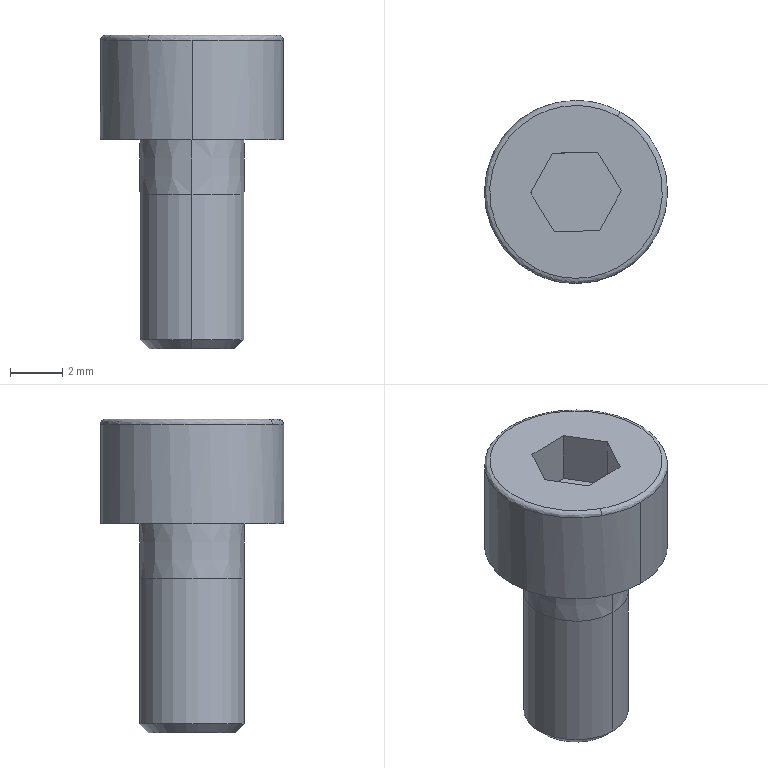Part | SolidWorks | features BaseBody 1 | 1 solid | 20 faces | box 7 x 7 x 12 mm | volume 237.96 mm3 | plane 10 | cylinder 4 | cone 4 | spline 2 | commonest cylinder face diameters 4 x2 7 x2
STEP:
#1=CARTESIAN_POINT('',(487.586,-57.42,293.048));
#2=VERTEX_POINT('',#1);
#3=CARTESIAN_POINT('',(489.266,-50.849,293.048));
#4=VERTEX_POINT('',#3);
#5=CARTESIAN_POINT('',(489.266,-54.349,293.048));
#6=DIRECTION('',(-0.000000004,0.000000009,-1.));
#7=DIRECTION('',(0.,1.,0.000000009));
#8=AXIS2_PLACEMENT_3D('',#5,#6,#7);
#9=CIRCLE('',#8,3.5);
#10=EDGE_CURVE('',#2,#4,#9,.T.);
#11=ORIENTED_EDGE('',*,*,#10,.F.);
#12=CARTESIAN_POINT('',(487.682,-57.244,293.248));
#13=VERTEX_POINT('',#12);
#14=CARTESIAN_POINT('',(487.682,-57.244,293.048));
#15=DIRECTION('',(-0.8773,0.4799,0.000000008));
#16=DIRECTION('',(-0.4799,-0.8773,-0.000000006));
#17=AXIS2_PLACEMENT_3D('',#14,#15,#16);
#18=CIRCLE('',#17,0.2);
#19=EDGE_CURVE('',#2,#13,#18,.T.);
#20=ORIENTED_EDGE('',*,*,#19,.T.);
#21=CARTESIAN_POINT('',(490.85,-51.454,293.248));
#22=VERTEX_POINT('',#21);
#23=CARTESIAN_POINT('',(487.682,-57.244,293.248));
#24=CARTESIAN_POINT('',(481.892,-54.077,293.248));
#25=CARTESIAN_POINT('',(485.059,-48.287,293.248));
#26=CARTESIAN_POINT('',(490.85,-51.454,293.248));
#27=(BOUNDED_CURVE()B_SPLINE_CURVE(3,(#23,#24,#25,#26),.UNSPECIFIED.,.F.,.F.)B_SPLINE_CURVE_WITH_KNOTS((4,4),(0.,1.),.UNSPECIFIED.)CURVE()GEOMETRIC_REPRESENTATION_ITEM()RATIONAL_B_SPLINE_CURVE((1.,0.3333,0.3333,1.))REPRESENTATION_ITEM(''));
#28=EDGE_CURVE('',#13,#22,#27,.T.);
#29=ORIENTED_EDGE('',*,*,#28,.T.);
#30=CARTESIAN_POINT('',(490.946,-51.279,293.048));
#31=VERTEX_POINT('',#30);
#32=CARTESIAN_POINT('',(490.85,-51.454,293.048));
#33=DIRECTION('',(0.8773,-0.4799,-0.000000008));
#34=DIRECTION('',(0.4799,0.8773,0.000000006));
#35=AXIS2_PLACEMENT_3D('',#32,#33,#34);
#36=CIRCLE('',#35,0.2);
#37=EDGE_CURVE('',#31,#22,#36,.T.);
#38=ORIENTED_EDGE('',*,*,#37,.F.);
#39=CARTESIAN_POINT('',(489.266,-54.349,293.048));
#40=DIRECTION('',(-0.000000004,0.000000009,-1.));
#41=DIRECTION('',(0.,1.,0.000000009));
#42=AXIS2_PLACEMENT_3D('',#39,#40,#41);
#43=CIRCLE('',#42,3.5);
#44=EDGE_CURVE('',#4,#31,#43,.T.);
#45=ORIENTED_EDGE('',*,*,#44,.F.);
#46=EDGE_LOOP('',(#11,#20,#29,#38,#45));
#47=FACE_OUTER_BOUND('',#46,.T.);
#48=CARTESIAN_POINT('',(487.586,-57.42,293.048));
#49=CARTESIAN_POINT('',(481.445,-54.06,293.048));
#50=CARTESIAN_POINT('',(484.804,-47.919,293.048));
#51=CARTESIAN_POINT('',(490.946,-51.279,293.048));
#52=CARTESIAN_POINT('',(487.586,-57.42,293.165));
#53=CARTESIAN_POINT('',(481.445,-54.06,293.165));
#54=CARTESIAN_POINT('',(484.804,-47.919,293.165));
#55=CARTESIAN_POINT('',(490.946,-51.279,293.165));
#56=CARTESIAN_POINT('',(487.626,-57.347,293.248));
#57=CARTESIAN_POINT('',(481.63,-54.067,293.248));
#58=CARTESIAN_POINT('',(484.91,-48.071,293.248));
#59=CARTESIAN_POINT('',(490.906,-51.351,293.248));
#60=CARTESIAN_POINT('',(487.682,-57.244,293.248));
#61=CARTESIAN_POINT('',(481.892,-54.077,293.248));
#62=CARTESIAN_POINT('',(485.059,-48.287,293.248));
#63=CARTESIAN_POINT('',(490.85,-51.454,293.248));
#64=(BOUNDED_SURFACE()B_SPLINE_SURFACE(3,3,((#48,#49,#50,#51),(#52,#53,#54,#55),(#56,#57,#58,#59),(#60,#61,#62,#63)),.UNSPECIFIED.,.F.,.F.,.T.)B_SPLINE_SURFACE_WITH_KNOTS((4,4),(4,4),(0.,1.),(0.,1.),.UNSPECIFIED.)GEOMETRIC_REPRESENTATION_ITEM()RATIONAL_B_SPLINE_SURFACE(((1.,0.3333,0.3333,1.),(0.8047,0.2682,0.2682,0.8047),(0.8047,0.2682,0.2682,0.8047),(1.,0.3333,0.3333,1.)))REPRESENTATION_ITEM('')SURFACE());
#65=ADVANCED_FACE('',(#47),#64,.T.);
#66=ORIENTED_EDGE('',*,*,#44,.T.);
#67=CARTESIAN_POINT('',(489.266,-57.849,293.048));
#68=VERTEX_POINT('',#67);
#69=CARTESIAN_POINT('',(489.266,-54.349,293.048));
#70=DIRECTION('',(-0.000000004,0.000000009,-1.));
#71=DIRECTION('',(0.,1.,0.000000009));
#72=AXIS2_PLACEMENT_3D('',#69,#70,#71);
#73=CIRCLE('',#72,3.5);
#74=EDGE_CURVE('',#31,#68,#73,.T.);
#75=ORIENTED_EDGE('',*,*,#74,.T.);
#76=CARTESIAN_POINT('',(489.266,-57.849,289.248));
#77=VERTEX_POINT('',#76);
#78=CARTESIAN_POINT('',(489.266,-57.849,291.148));
#79=DIRECTION('',(-0.000000004,0.000000009,-1.));
#80=VECTOR('',#79,1000.);
#81=LINE('',#78,#80);
#82=EDGE_CURVE('',#68,#77,#81,.T.);
#83=ORIENTED_EDGE('',*,*,#82,.T.);
#84=CARTESIAN_POINT('',(489.266,-50.849,289.248));
#85=VERTEX_POINT('',#84);
#86=CARTESIAN_POINT('',(489.266,-54.349,289.248));
#87=DIRECTION('',(0.000000004,-0.000000009,1.));
#88=DIRECTION('',(0.,1.,0.000000009));
#89=AXIS2_PLACEMENT_3D('',#86,#87,#88);
#90=CIRCLE('',#89,3.5);
#91=EDGE_CURVE('',#77,#85,#90,.T.);
#92=ORIENTED_EDGE('',*,*,#91,.T.);
#93=CARTESIAN_POINT('',(489.266,-50.849,291.148));
#94=DIRECTION('',(-0.000000004,0.000000009,-1.));
#95=VECTOR('',#94,1000.);
#96=LINE('',#93,#95);
#97=EDGE_CURVE('',#4,#85,#96,.T.);
#98=ORIENTED_EDGE('',*,*,#97,.F.);
#99=EDGE_LOOP('',(#66,#75,#83,#92,#98));
#100=FACE_OUTER_BOUND('',#99,.T.);
#101=CARTESIAN_POINT('',(489.266,-54.349,291.148));
#102=DIRECTION('',(-0.000000004,0.000000009,-1.));
#103=DIRECTION('',(0.,1.,0.000000009));
#104=AXIS2_PLACEMENT_3D('',#101,#102,#103);
#105=CYLINDRICAL_SURFACE('',#104,3.5);
#106=ADVANCED_FACE('',(#100),#105,.T.);
#107=CARTESIAN_POINT('',(489.266,-56.348,289.248));
#108=VERTEX_POINT('',#107);
#109=CARTESIAN_POINT('',(489.266,-52.35,289.248));
#110=VERTEX_POINT('',#109);
#111=CARTESIAN_POINT('',(489.266,-54.349,289.248));
#112=DIRECTION('',(0.000000004,-0.000000009,1.));
#113=DIRECTION('',(0.,1.,0.000000009));
#114=AXIS2_PLACEMENT_3D('',#111,#112,#113);
#115=CIRCLE('',#114,1.999);
#116=EDGE_CURVE('',#108,#110,#115,.T.);
#117=ORIENTED_EDGE('',*,*,#116,.F.);
#118=CARTESIAN_POINT('',(489.266,-56.349,287.148));
#119=VERTEX_POINT('',#118);
#120=CARTESIAN_POINT('',(489.266,-56.349,287.148));
#121=DIRECTION('',(-0.000000004,-0.0004762,-1.));
#122=VECTOR('',#121,1000.);
#123=LINE('',#120,#122);
#124=EDGE_CURVE('',#108,#119,#123,.T.);
#125=ORIENTED_EDGE('',*,*,#124,.T.);
#126=CARTESIAN_POINT('',(489.266,-52.349,287.148));
#127=VERTEX_POINT('',#126);
#128=CARTESIAN_POINT('',(489.266,-54.349,287.148));
#129=DIRECTION('',(0.000000004,-0.000000009,1.));
#130=DIRECTION('',(0.4799,0.8773,0.000000006));
#131=AXIS2_PLACEMENT_3D('',#128,#129,#130);
#132=CIRCLE('',#131,2.);
#133=EDGE_CURVE('',#119,#127,#132,.T.);
#134=ORIENTED_EDGE('',*,*,#133,.T.);
#135=CARTESIAN_POINT('',(489.266,-52.349,287.148));
#136=DIRECTION('',(-0.000000004,0.0004762,-1.));
#137=VECTOR('',#136,1000.);
#138=LINE('',#135,#137);
#139=EDGE_CURVE('',#110,#127,#138,.T.);
#140=ORIENTED_EDGE('',*,*,#139,.F.);
#141=EDGE_LOOP('',(#117,#125,#134,#140));
#142=FACE_OUTER_BOUND('',#141,.T.);
#143=CARTESIAN_POINT('',(489.266,-54.349,287.148));
#144=DIRECTION('',(-0.000000004,0.000000009,-1.));
#145=DIRECTION('',(0.,1.,0.000000009));
#146=AXIS2_PLACEMENT_3D('',#143,#144,#145);
#147=CONICAL_SURFACE('',#146,2.,0.0004762);
#148=ADVANCED_FACE('',(#142),#147,.T.);
#149=ORIENTED_EDGE('',*,*,#133,.F.);
#150=CARTESIAN_POINT('',(489.266,-56.349,281.598));
#151=VERTEX_POINT('',#150);
#152=CARTESIAN_POINT('',(489.266,-56.349,284.373));
#153=DIRECTION('',(-0.000000004,0.000000009,-1.));
#154=VECTOR('',#153,1000.);
#155=LINE('',#152,#154);
#156=EDGE_CURVE('',#119,#151,#155,.T.);
#157=ORIENTED_EDGE('',*,*,#156,.T.);
#158=CARTESIAN_POINT('',(489.266,-52.349,281.598));
#159=VERTEX_POINT('',#158);
#160=CARTESIAN_POINT('',(489.266,-54.349,281.598));
#161=DIRECTION('',(0.000000004,-0.000000009,1.));
#162=DIRECTION('',(0.,1.,0.000000009));
#163=AXIS2_PLACEMENT_3D('',#160,#161,#162);
#164=CIRCLE('',#163,2.);
#165=EDGE_CURVE('',#151,#159,#164,.T.);
#166=ORIENTED_EDGE('',*,*,#165,.T.);
#167=CARTESIAN_POINT('',(489.266,-52.349,284.373));
#168=DIRECTION('',(-0.000000004,0.000000009,-1.));
#169=VECTOR('',#168,1000.);
#170=LINE('',#167,#169);
#171=EDGE_CURVE('',#127,#159,#170,.T.);
#172=ORIENTED_EDGE('',*,*,#171,.F.);
#173=EDGE_LOOP('',(#149,#157,#166,#172));
#174=FACE_OUTER_BOUND('',#173,.T.);
#175=CARTESIAN_POINT('',(489.266,-54.349,284.373));
#176=DIRECTION('',(-0.000000004,0.000000009,-1.));
#177=DIRECTION('',(0.,1.,0.000000009));
#178=AXIS2_PLACEMENT_3D('',#175,#176,#177);
#179=CYLINDRICAL_SURFACE('',#178,2.);
#180=ADVANCED_FACE('',(#174),#179,.T.);
#181=CARTESIAN_POINT('',(489.266,-55.999,281.248));
#182=VERTEX_POINT('',#181);
#183=CARTESIAN_POINT('',(489.266,-52.699,281.248));
#184=VERTEX_POINT('',#183);
#185=CARTESIAN_POINT('',(489.266,-54.349,281.248));
#186=DIRECTION('',(0.000000004,-0.000000009,1.));
#187=DIRECTION('',(0.,-1.,-0.000000009));
#188=AXIS2_PLACEMENT_3D('',#185,#186,#187);
#189=CIRCLE('',#188,1.65);
#190=EDGE_CURVE('',#182,#184,#189,.T.);
#191=ORIENTED_EDGE('',*,*,#190,.T.);
#192=CARTESIAN_POINT('',(489.266,-52.349,281.598));
#193=DIRECTION('',(0.000000003,0.7071,0.7071));
#194=VECTOR('',#193,1000.);
#195=LINE('',#192,#194);
#196=EDGE_CURVE('',#184,#159,#195,.T.);
#197=ORIENTED_EDGE('',*,*,#196,.T.);
#198=ORIENTED_EDGE('',*,*,#165,.F.);
#199=CARTESIAN_POINT('',(489.266,-56.349,281.598));
#200=DIRECTION('',(0.000000003,-0.7071,0.7071));
#201=VECTOR('',#200,1000.);
#202=LINE('',#199,#201);
#203=EDGE_CURVE('',#182,#151,#202,.T.);
#204=ORIENTED_EDGE('',*,*,#203,.F.);
#205=EDGE_LOOP('',(#191,#197,#198,#204));
#206=FACE_OUTER_BOUND('',#205,.T.);
#207=CARTESIAN_POINT('',(489.266,-54.349,281.598));
#208=DIRECTION('',(0.000000004,-0.000000009,1.));
#209=DIRECTION('',(0.,-1.,-0.000000009));
#210=AXIS2_PLACEMENT_3D('',#207,#208,#209);
#211=CONICAL_SURFACE('',#210,2.,0.7854);
#212=ADVANCED_FACE('',(#206),#211,.T.);
#213=ORIENTED_EDGE('',*,*,#82,.F.);
#214=CARTESIAN_POINT('',(489.266,-54.349,293.048));
#215=DIRECTION('',(-0.000000004,0.000000009,-1.));
#216=DIRECTION('',(0.,1.,0.000000009));
#217=AXIS2_PLACEMENT_3D('',#214,#215,#216);
#218=CIRCLE('',#217,3.5);
#219=EDGE_CURVE('',#68,#2,#218,.T.);
#220=ORIENTED_EDGE('',*,*,#219,.T.);
#221=ORIENTED_EDGE('',*,*,#10,.T.);
#222=ORIENTED_EDGE('',*,*,#97,.T.);
#223=CARTESIAN_POINT('',(489.266,-54.349,289.248));
#224=DIRECTION('',(0.000000004,-0.000000009,1.));
#225=DIRECTION('',(0.,1.,0.000000009));
#226=AXIS2_PLACEMENT_3D('',#223,#224,#225);
#227=CIRCLE('',#226,3.5);
#228=EDGE_CURVE('',#85,#77,#227,.T.);
#229=ORIENTED_EDGE('',*,*,#228,.T.);
#230=EDGE_LOOP('',(#213,#220,#221,#222,#229));
#231=FACE_OUTER_BOUND('',#230,.T.);
#232=CARTESIAN_POINT('',(489.266,-54.349,291.148));
#233=DIRECTION('',(-0.000000004,0.000000009,-1.));
#234=DIRECTION('',(0.,1.,0.000000009));
#235=AXIS2_PLACEMENT_3D('',#232,#233,#234);
#236=CYLINDRICAL_SURFACE('',#235,3.5);
#237=ADVANCED_FACE('',(#231),#236,.T.);
#238=CARTESIAN_POINT('',(489.266,-54.349,289.248));
#239=DIRECTION('',(0.000000004,-0.000000009,1.));
#240=DIRECTION('',(0.,1.,0.000000009));
#241=AXIS2_PLACEMENT_3D('',#238,#239,#240);
#242=CIRCLE('',#241,1.999);
#243=EDGE_CURVE('',#110,#108,#242,.T.);
#244=ORIENTED_EDGE('',*,*,#243,.T.);
#245=ORIENTED_EDGE('',*,*,#116,.T.);
#246=EDGE_LOOP('',(#244,#245));
#247=FACE_BOUND('',#246,.T.);
#248=ORIENTED_EDGE('',*,*,#228,.F.);
#249=ORIENTED_EDGE('',*,*,#91,.F.);
#250=EDGE_LOOP('',(#248,#249));
#251=FACE_OUTER_BOUND('',#250,.T.);
#252=CARTESIAN_POINT('',(490.106,-52.814,289.248));
#253=DIRECTION('',(-0.000000004,0.000000009,-1.));
#254=DIRECTION('',(0.,1.,0.000000009));
#255=AXIS2_PLACEMENT_3D('',#252,#253,#254);
#256=PLANE('',#255);
#257=ADVANCED_FACE('',(#247,#251),#256,.T.);
#258=ORIENTED_EDGE('',*,*,#19,.F.);
#259=ORIENTED_EDGE('',*,*,#219,.F.);
#260=ORIENTED_EDGE('',*,*,#74,.F.);
#261=ORIENTED_EDGE('',*,*,#37,.T.);
#262=CARTESIAN_POINT('',(490.85,-51.454,293.248));
#263=CARTESIAN_POINT('',(496.64,-54.621,293.248));
#264=CARTESIAN_POINT('',(493.472,-60.412,293.248));
#265=CARTESIAN_POINT('',(487.682,-57.244,293.248));
#266=(BOUNDED_CURVE()B_SPLINE_CURVE(3,(#262,#263,#264,#265),.UNSPECIFIED.,.F.,.F.)B_SPLINE_CURVE_WITH_KNOTS((4,4),(0.,1.),.UNSPECIFIED.)CURVE()GEOMETRIC_REPRESENTATION_ITEM()RATIONAL_B_SPLINE_CURVE((1.,0.3333,0.3333,1.))REPRESENTATION_ITEM(''));
#267=EDGE_CURVE('',#22,#13,#266,.T.);
#268=ORIENTED_EDGE('',*,*,#267,.T.);
#269=EDGE_LOOP('',(#258,#259,#260,#261,#268));
#270=FACE_OUTER_BOUND('',#269,.T.);
#271=CARTESIAN_POINT('',(490.946,-51.279,293.048));
#272=CARTESIAN_POINT('',(497.087,-54.638,293.048));
#273=CARTESIAN_POINT('',(493.727,-60.779,293.048));
#274=CARTESIAN_POINT('',(487.586,-57.42,293.048));
#275=CARTESIAN_POINT('',(490.946,-51.279,293.165));
#276=CARTESIAN_POINT('',(497.087,-54.638,293.165));
#277=CARTESIAN_POINT('',(493.727,-60.779,293.165));
#278=CARTESIAN_POINT('',(487.586,-57.42,293.165));
#279=CARTESIAN_POINT('',(490.906,-51.351,293.248));
#280=CARTESIAN_POINT('',(496.902,-54.631,293.248));
#281=CARTESIAN_POINT('',(493.622,-60.627,293.248));
#282=CARTESIAN_POINT('',(487.626,-57.347,293.248));
#283=CARTESIAN_POINT('',(490.85,-51.454,293.248));
#284=CARTESIAN_POINT('',(496.64,-54.621,293.248));
#285=CARTESIAN_POINT('',(493.472,-60.412,293.248));
#286=CARTESIAN_POINT('',(487.682,-57.244,293.248));
#287=(BOUNDED_SURFACE()B_SPLINE_SURFACE(3,3,((#271,#272,#273,#274),(#275,#276,#277,#278),(#279,#280,#281,#282),(#283,#284,#285,#286)),.UNSPECIFIED.,.F.,.F.,.F.)B_SPLINE_SURFACE_WITH_KNOTS((4,4),(4,4),(0.,1.),(0.,1.),.UNSPECIFIED.)GEOMETRIC_REPRESENTATION_ITEM()RATIONAL_B_SPLINE_SURFACE(((1.,0.3333,0.3333,1.),(0.8047,0.2682,0.2682,0.8047),(0.8047,0.2682,0.2682,0.8047),(1.,0.3333,0.3333,1.)))REPRESENTATION_ITEM('')SURFACE());
#288=ADVANCED_FACE('',(#270),#287,.T.);
#289=ORIENTED_EDGE('',*,*,#124,.F.);
#290=ORIENTED_EDGE('',*,*,#243,.F.);
#291=ORIENTED_EDGE('',*,*,#139,.T.);
#292=CARTESIAN_POINT('',(489.266,-54.349,287.148));
#293=DIRECTION('',(0.000000004,-0.000000009,1.));
#294=DIRECTION('',(0.4799,0.8773,0.000000006));
#295=AXIS2_PLACEMENT_3D('',#292,#293,#294);
#296=CIRCLE('',#295,2.);
#297=EDGE_CURVE('',#127,#119,#296,.T.);
#298=ORIENTED_EDGE('',*,*,#297,.T.);
#299=EDGE_LOOP('',(#289,#290,#291,#298));
#300=FACE_OUTER_BOUND('',#299,.T.);
#301=CARTESIAN_POINT('',(489.266,-54.349,287.148));
#302=DIRECTION('',(-0.000000004,0.000000009,-1.));
#303=DIRECTION('',(0.,1.,0.000000009));
#304=AXIS2_PLACEMENT_3D('',#301,#302,#303);
#305=CONICAL_SURFACE('',#304,2.,0.0004762);
#306=ADVANCED_FACE('',(#300),#305,.T.);
#307=ORIENTED_EDGE('',*,*,#28,.F.);
#308=ORIENTED_EDGE('',*,*,#267,.F.);
#309=EDGE_LOOP('',(#307,#308));
#310=FACE_OUTER_BOUND('',#309,.T.);
#311=CARTESIAN_POINT('',(490.166,-55.829,293.248));
#312=VERTEX_POINT('',#311);
#313=CARTESIAN_POINT('',(488.435,-55.869,293.248));
#314=VERTEX_POINT('',#313);
#315=CARTESIAN_POINT('',(488.435,-55.869,293.248));
#316=DIRECTION('',(-0.9997,-0.02304,0.));
#317=VECTOR('',#316,1000.);
#318=LINE('',#315,#317);
#319=EDGE_CURVE('',#312,#314,#318,.T.);
#320=ORIENTED_EDGE('',*,*,#319,.T.);
#321=CARTESIAN_POINT('',(487.534,-54.389,293.248));
#322=VERTEX_POINT('',#321);
#323=CARTESIAN_POINT('',(488.435,-55.869,293.248));
#324=DIRECTION('',(-0.5198,0.8543,0.000000009));
#325=VECTOR('',#324,1000.);
#326=LINE('',#323,#325);
#327=EDGE_CURVE('',#314,#322,#326,.T.);
#328=ORIENTED_EDGE('',*,*,#327,.T.);
#329=CARTESIAN_POINT('',(488.366,-52.87,293.248));
#330=VERTEX_POINT('',#329);
#331=CARTESIAN_POINT('',(488.366,-52.87,293.248));
#332=DIRECTION('',(0.4799,0.8773,0.));
#333=VECTOR('',#332,1000.);
#334=LINE('',#331,#333);
#335=EDGE_CURVE('',#322,#330,#334,.T.);
#336=ORIENTED_EDGE('',*,*,#335,.T.);
#337=CARTESIAN_POINT('',(490.097,-52.83,293.248));
#338=VERTEX_POINT('',#337);
#339=CARTESIAN_POINT('',(490.097,-52.83,293.248));
#340=DIRECTION('',(0.9997,0.02304,0.));
#341=VECTOR('',#340,1000.);
#342=LINE('',#339,#341);
#343=EDGE_CURVE('',#330,#338,#342,.T.);
#344=ORIENTED_EDGE('',*,*,#343,.T.);
#345=CARTESIAN_POINT('',(490.997,-54.309,293.248));
#346=VERTEX_POINT('',#345);
#347=CARTESIAN_POINT('',(490.997,-54.309,293.248));
#348=DIRECTION('',(0.5198,-0.8543,0.));
#349=VECTOR('',#348,1000.);
#350=LINE('',#347,#349);
#351=EDGE_CURVE('',#338,#346,#350,.T.);
#352=ORIENTED_EDGE('',*,*,#351,.T.);
#353=CARTESIAN_POINT('',(490.166,-55.829,293.248));
#354=DIRECTION('',(-0.4799,-0.8773,0.));
#355=VECTOR('',#354,1000.);
#356=LINE('',#353,#355);
#357=EDGE_CURVE('',#346,#312,#356,.T.);
#358=ORIENTED_EDGE('',*,*,#357,.T.);
#359=EDGE_LOOP('',(#320,#328,#336,#344,#352,#358));
#360=FACE_BOUND('',#359,.T.);
#361=CARTESIAN_POINT('',(490.058,-52.902,293.248));
#362=DIRECTION('',(0.000000004,-0.000000009,1.));
#363=DIRECTION('',(0.,-1.,-0.000000009));
#364=AXIS2_PLACEMENT_3D('',#361,#362,#363);
#365=PLANE('',#364);
#366=ADVANCED_FACE('',(#310,#360),#365,.T.);
#367=ORIENTED_EDGE('',*,*,#156,.F.);
#368=ORIENTED_EDGE('',*,*,#297,.F.);
#369=ORIENTED_EDGE('',*,*,#171,.T.);
#370=CARTESIAN_POINT('',(489.266,-54.349,281.598));
#371=DIRECTION('',(0.000000004,-0.000000009,1.));
#372=DIRECTION('',(0.,1.,0.000000009));
#373=AXIS2_PLACEMENT_3D('',#370,#371,#372);
#374=CIRCLE('',#373,2.);
#375=EDGE_CURVE('',#159,#151,#374,.T.);
#376=ORIENTED_EDGE('',*,*,#375,.T.);
#377=EDGE_LOOP('',(#367,#368,#369,#376));
#378=FACE_OUTER_BOUND('',#377,.T.);
#379=CARTESIAN_POINT('',(489.266,-54.349,284.373));
#380=DIRECTION('',(-0.000000004,0.000000009,-1.));
#381=DIRECTION('',(0.,1.,0.000000009));
#382=AXIS2_PLACEMENT_3D('',#379,#380,#381);
#383=CYLINDRICAL_SURFACE('',#382,2.);
#384=ADVANCED_FACE('',(#378),#383,.T.);
#385=CARTESIAN_POINT('',(487.534,-54.389,291.248));
#386=VERTEX_POINT('',#385);
#387=CARTESIAN_POINT('',(487.534,-54.389,293.248));
#388=DIRECTION('',(0.000000001,0.000000001,-1.));
#389=VECTOR('',#388,1000.);
#390=LINE('',#387,#389);
#391=EDGE_CURVE('',#322,#386,#390,.T.);
#392=ORIENTED_EDGE('',*,*,#391,.F.);
#393=ORIENTED_EDGE('',*,*,#327,.F.);
#394=CARTESIAN_POINT('',(488.435,-55.869,291.248));
#395=VERTEX_POINT('',#394);
#396=CARTESIAN_POINT('',(488.435,-55.869,293.248));
#397=DIRECTION('',(-0.000000001,-0.000000001,1.));
#398=VECTOR('',#397,1000.);
#399=LINE('',#396,#398);
#400=EDGE_CURVE('',#395,#314,#399,.T.);
#401=ORIENTED_EDGE('',*,*,#400,.F.);
#402=CARTESIAN_POINT('',(487.534,-54.389,291.248));
#403=DIRECTION('',(0.5198,-0.8543,0.));
#404=VECTOR('',#403,1000.);
#405=LINE('',#402,#404);
#406=EDGE_CURVE('',#386,#395,#405,.T.);
#407=ORIENTED_EDGE('',*,*,#406,.F.);
#408=EDGE_LOOP('',(#392,#393,#401,#407));
#409=FACE_OUTER_BOUND('',#408,.T.);
#410=CARTESIAN_POINT('',(487.534,-54.389,293.248));
#411=DIRECTION('',(-0.8543,-0.5198,-0.000000001));
#412=DIRECTION('',(0.5198,-0.8543,0.));
#413=AXIS2_PLACEMENT_3D('',#410,#411,#412);
#414=PLANE('',#413);
#415=ADVANCED_FACE('',(#409),#414,.F.);
#416=ORIENTED_EDGE('',*,*,#196,.F.);
#417=CARTESIAN_POINT('',(489.266,-54.349,281.248));
#418=DIRECTION('',(0.000000004,-0.000000009,1.));
#419=DIRECTION('',(0.,-1.,-0.000000009));
#420=AXIS2_PLACEMENT_3D('',#417,#418,#419);
#421=CIRCLE('',#420,1.65);
#422=EDGE_CURVE('',#184,#182,#421,.T.);
#423=ORIENTED_EDGE('',*,*,#422,.T.);
#424=ORIENTED_EDGE('',*,*,#203,.T.);
#425=ORIENTED_EDGE('',*,*,#375,.F.);
#426=EDGE_LOOP('',(#416,#423,#424,#425));
#427=FACE_OUTER_BOUND('',#426,.T.);
#428=CARTESIAN_POINT('',(489.266,-54.349,281.598));
#429=DIRECTION('',(0.000000004,-0.000000009,1.));
#430=DIRECTION('',(0.,-1.,-0.000000009));
#431=AXIS2_PLACEMENT_3D('',#428,#429,#430);
#432=CONICAL_SURFACE('',#431,2.,0.7854);
#433=ADVANCED_FACE('',(#427),#432,.T.);
#434=CARTESIAN_POINT('',(490.997,-54.309,291.248));
#435=VERTEX_POINT('',#434);
#436=CARTESIAN_POINT('',(490.097,-52.83,291.248));
#437=VERTEX_POINT('',#436);
#438=CARTESIAN_POINT('',(490.997,-54.309,291.248));
#439=DIRECTION('',(-0.5198,0.8543,0.));
#440=VECTOR('',#439,1000.);
#441=LINE('',#438,#440);
#442=EDGE_CURVE('',#435,#437,#441,.T.);
#443=ORIENTED_EDGE('',*,*,#442,.T.);
#444=CARTESIAN_POINT('',(488.366,-52.87,291.248));
#445=VERTEX_POINT('',#444);
#446=CARTESIAN_POINT('',(490.097,-52.83,291.248));
#447=DIRECTION('',(-0.9997,-0.02304,0.));
#448=VECTOR('',#447,1000.);
#449=LINE('',#446,#448);
#450=EDGE_CURVE('',#437,#445,#449,.T.);
#451=ORIENTED_EDGE('',*,*,#450,.T.);
#452=CARTESIAN_POINT('',(488.366,-52.87,291.248));
#453=DIRECTION('',(-0.4799,-0.8773,-0.000000006));
#454=VECTOR('',#453,1000.);
#455=LINE('',#452,#454);
#456=EDGE_CURVE('',#445,#386,#455,.T.);
#457=ORIENTED_EDGE('',*,*,#456,.T.);
#458=ORIENTED_EDGE('',*,*,#406,.T.);
#459=CARTESIAN_POINT('',(490.166,-55.829,291.248));
#460=VERTEX_POINT('',#459);
#461=CARTESIAN_POINT('',(488.435,-55.869,291.248));
#462=DIRECTION('',(0.9997,0.02304,-0.000000004));
#463=VECTOR('',#462,1000.);
#464=LINE('',#461,#463);
#465=EDGE_CURVE('',#395,#460,#464,.T.);
#466=ORIENTED_EDGE('',*,*,#465,.T.);
#467=CARTESIAN_POINT('',(490.166,-55.829,291.248));
#468=DIRECTION('',(0.4799,0.8773,0.));
#469=VECTOR('',#468,1000.);
#470=LINE('',#467,#469);
#471=EDGE_CURVE('',#460,#435,#470,.T.);
#472=ORIENTED_EDGE('',*,*,#471,.T.);
#473=EDGE_LOOP('',(#443,#451,#457,#458,#466,#472));
#474=FACE_OUTER_BOUND('',#473,.T.);
#475=CARTESIAN_POINT('',(489.266,-54.349,291.248));
#476=DIRECTION('',(0.000000004,-0.000000009,1.));
#477=DIRECTION('',(0.,-1.,-0.000000009));
#478=AXIS2_PLACEMENT_3D('',#475,#476,#477);
#479=PLANE('',#478);
#480=ADVANCED_FACE('',(#474),#479,.T.);
#481=CARTESIAN_POINT('',(488.366,-52.87,293.248));
#482=DIRECTION('',(-0.000000007,0.000000004,-1.));
#483=VECTOR('',#482,1000.);
#484=LINE('',#481,#483);
#485=EDGE_CURVE('',#330,#445,#484,.T.);
#486=ORIENTED_EDGE('',*,*,#485,.F.);
#487=ORIENTED_EDGE('',*,*,#335,.F.);
#488=ORIENTED_EDGE('',*,*,#391,.T.);
#489=ORIENTED_EDGE('',*,*,#456,.F.);
#490=EDGE_LOOP('',(#486,#487,#488,#489));
#491=FACE_OUTER_BOUND('',#490,.T.);
#492=CARTESIAN_POINT('',(488.366,-52.87,293.248));
#493=DIRECTION('',(-0.8773,0.4799,0.000000008));
#494=DIRECTION('',(-0.4799,-0.8773,0.));
#495=AXIS2_PLACEMENT_3D('',#492,#493,#494);
#496=PLANE('',#495);
#497=ADVANCED_FACE('',(#491),#496,.F.);
#498=ORIENTED_EDGE('',*,*,#400,.T.);
#499=ORIENTED_EDGE('',*,*,#319,.F.);
#500=CARTESIAN_POINT('',(490.166,-55.829,293.248));
#501=DIRECTION('',(0.,-0.000000009,1.));
#502=VECTOR('',#501,1000.);
#503=LINE('',#500,#502);
#504=EDGE_CURVE('',#460,#312,#503,.T.);
#505=ORIENTED_EDGE('',*,*,#504,.F.);
#506=ORIENTED_EDGE('',*,*,#465,.F.);
#507=EDGE_LOOP('',(#498,#499,#505,#506));
#508=FACE_OUTER_BOUND('',#507,.T.);
#509=CARTESIAN_POINT('',(488.435,-55.869,293.248));
#510=DIRECTION('',(0.02304,-0.9997,-0.000000009));
#511=DIRECTION('',(0.9997,0.02304,0.));
#512=AXIS2_PLACEMENT_3D('',#509,#510,#511);
#513=PLANE('',#512);
#514=ADVANCED_FACE('',(#508),#513,.F.);
#515=ORIENTED_EDGE('',*,*,#190,.F.);
#516=ORIENTED_EDGE('',*,*,#422,.F.);
#517=EDGE_LOOP('',(#515,#516));
#518=FACE_OUTER_BOUND('',#517,.T.);
#519=CARTESIAN_POINT('',(489.662,-53.625,281.248));
#520=DIRECTION('',(-0.000000004,0.000000009,-1.));
#521=DIRECTION('',(0.,1.,0.000000009));
#522=AXIS2_PLACEMENT_3D('',#519,#520,#521);
#523=PLANE('',#522);
#524=ADVANCED_FACE('',(#518),#523,.T.);
#525=CARTESIAN_POINT('',(490.097,-52.83,293.248));
#526=DIRECTION('',(0.,0.000000009,-1.));
#527=VECTOR('',#526,1000.);
#528=LINE('',#525,#527);
#529=EDGE_CURVE('',#338,#437,#528,.T.);
#530=ORIENTED_EDGE('',*,*,#529,.F.);
#531=ORIENTED_EDGE('',*,*,#343,.F.);
#532=ORIENTED_EDGE('',*,*,#485,.T.);
#533=ORIENTED_EDGE('',*,*,#450,.F.);
#534=EDGE_LOOP('',(#530,#531,#532,#533));
#535=FACE_OUTER_BOUND('',#534,.T.);
#536=CARTESIAN_POINT('',(490.097,-52.83,293.248));
#537=DIRECTION('',(-0.02304,0.9997,0.000000009));
#538=DIRECTION('',(-0.9997,-0.02304,0.));
#539=AXIS2_PLACEMENT_3D('',#536,#537,#538);
#540=PLANE('',#539);
#541=ADVANCED_FACE('',(#535),#540,.F.);
#542=ORIENTED_EDGE('',*,*,#504,.T.);
#543=ORIENTED_EDGE('',*,*,#357,.F.);
#544=CARTESIAN_POINT('',(490.997,-54.309,293.248));
#545=DIRECTION('',(0.000000007,-0.000000004,1.));
#546=VECTOR('',#545,1000.);
#547=LINE('',#544,#546);
#548=EDGE_CURVE('',#435,#346,#547,.T.);
#549=ORIENTED_EDGE('',*,*,#548,.F.);
#550=ORIENTED_EDGE('',*,*,#471,.F.);
#551=EDGE_LOOP('',(#542,#543,#549,#550));
#552=FACE_OUTER_BOUND('',#551,.T.);
#553=CARTESIAN_POINT('',(490.166,-55.829,293.248));
#554=DIRECTION('',(0.8773,-0.4799,-0.000000008));
#555=DIRECTION('',(0.4799,0.8773,0.));
#556=AXIS2_PLACEMENT_3D('',#553,#554,#555);
#557=PLANE('',#556);
#558=ADVANCED_FACE('',(#552),#557,.F.);
#559=ORIENTED_EDGE('',*,*,#548,.T.);
#560=ORIENTED_EDGE('',*,*,#351,.F.);
#561=ORIENTED_EDGE('',*,*,#529,.T.);
#562=ORIENTED_EDGE('',*,*,#442,.F.);
#563=EDGE_LOOP('',(#559,#560,#561,#562));
#564=FACE_OUTER_BOUND('',#563,.T.);
#565=CARTESIAN_POINT('',(490.997,-54.309,293.248));
#566=DIRECTION('',(0.8543,0.5198,0.000000001));
#567=DIRECTION('',(-0.5198,0.8543,0.));
#568=AXIS2_PLACEMENT_3D('',#565,#566,#567);
#569=PLANE('',#568);
#570=ADVANCED_FACE('',(#564),#569,.F.);
#571=CLOSED_SHELL('',(#65,#106,#148,#180,#212,#237,#257,#288,#306,#366,#384,#415,#433,#480,#497,#514,#524,#541,#558,#570));
#572=MANIFOLD_SOLID_BREP('',#571);
#573=CARTESIAN_POINT('',(0.,0.,0.));
#574=DIRECTION('',(0.,0.,1.));
#575=DIRECTION('',(1.,0.,0.));
#576=AXIS2_PLACEMENT_3D('',#573,#574,#575);
#577=(LENGTH_UNIT()NAMED_UNIT(*)SI_UNIT(.MILLI.,.METRE.));
#578=UNCERTAINTY_MEASURE_WITH_UNIT(LENGTH_MEASURE(0.00001),#577,'','');
#579=(NAMED_UNIT(*)PLANE_ANGLE_UNIT()SI_UNIT($,.RADIAN.));
#580=(NAMED_UNIT(*)SI_UNIT($,.STERADIAN.)SOLID_ANGLE_UNIT());
#581=(GEOMETRIC_REPRESENTATION_CONTEXT(3)GLOBAL_UNCERTAINTY_ASSIGNED_CONTEXT((#578))GLOBAL_UNIT_ASSIGNED_CONTEXT((#577,#579,#580))REPRESENTATION_CONTEXT('',''));
#582=ADVANCED_BREP_SHAPE_REPRESENTATION('',(#572,#576),#581);